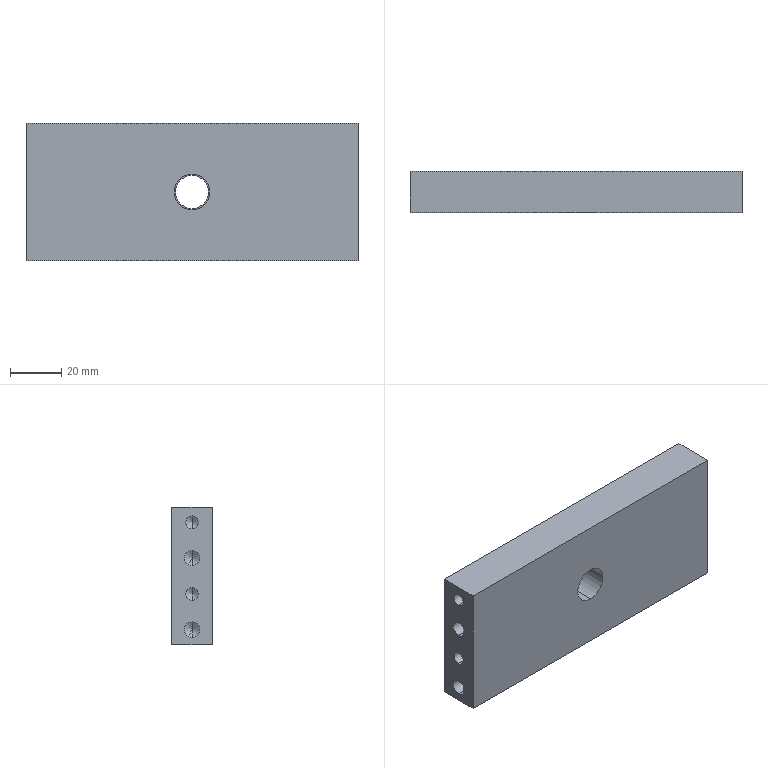Part | STEP file | OP10-154_inclined plate (L) | 1 solid | 59 faces | box 130 x 16 x 54 mm | volume 106815 mm3 | cylinder 28 | cone 24 | plane 7 | commonest cylinder face diameters 4.2 x8 5 x8 6 x8 13 x2 14 x2